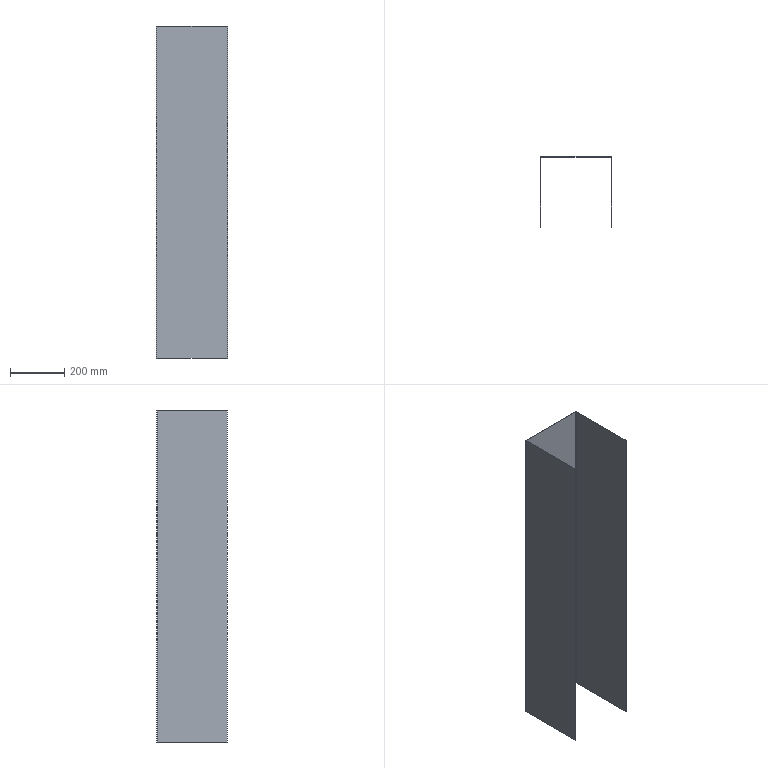Part | 1 solid | 22 faces | box 262 x 261 x 1225 mm | volume 956650 mm3 | plane 18 | cylinder 4 | commonest cylinder face diameters 1.473 x2 3.473 x2
STEP:
#1=CARTESIAN_POINT('',(129.263,260.,1225.));
#2=VERTEX_POINT('',#1);
#3=CARTESIAN_POINT('',(129.263,261.,1225.));
#4=VERTEX_POINT('',#3);
#5=CARTESIAN_POINT('',(129.263,260.,1225.));
#6=DIRECTION('',(0.,1.,0.));
#7=VECTOR('',#6,1000.);
#8=LINE('',#5,#7);
#9=EDGE_CURVE('',#2,#4,#8,.T.);
#10=ORIENTED_EDGE('',*,*,#9,.F.);
#11=CARTESIAN_POINT('',(130.,259.263,1225.));
#12=VERTEX_POINT('',#11);
#13=CARTESIAN_POINT('',(129.263,259.263,1225.));
#14=DIRECTION('',(0.,0.,1.));
#15=DIRECTION('',(-1.,0.,0.));
#16=AXIS2_PLACEMENT_3D('',#13,#14,#15);
#17=CIRCLE('',#16,0.7366);
#18=EDGE_CURVE('',#12,#2,#17,.T.);
#19=ORIENTED_EDGE('',*,*,#18,.F.);
#20=CARTESIAN_POINT('',(131.,259.263,1225.));
#21=VERTEX_POINT('',#20);
#22=CARTESIAN_POINT('',(131.,259.263,1225.));
#23=DIRECTION('',(-1.,0.,0.));
#24=VECTOR('',#23,1000.);
#25=LINE('',#22,#24);
#26=EDGE_CURVE('',#21,#12,#25,.T.);
#27=ORIENTED_EDGE('',*,*,#26,.F.);
#28=CARTESIAN_POINT('',(129.263,259.263,1225.));
#29=DIRECTION('',(0.,0.,1.));
#30=DIRECTION('',(1.,0.,0.));
#31=AXIS2_PLACEMENT_3D('',#28,#29,#30);
#32=CIRCLE('',#31,1.737);
#33=EDGE_CURVE('',#21,#4,#32,.T.);
#34=ORIENTED_EDGE('',*,*,#33,.T.);
#35=EDGE_LOOP('',(#10,#19,#27,#34));
#36=FACE_OUTER_BOUND('',#35,.T.);
#37=CARTESIAN_POINT('',(129.263,260.,1225.));
#38=DIRECTION('',(0.,0.,1.));
#39=DIRECTION('',(1.,0.,0.));
#40=AXIS2_PLACEMENT_3D('',#37,#38,#39);
#41=PLANE('',#40);
#42=ADVANCED_FACE('',(#36),#41,.T.);
#43=CARTESIAN_POINT('',(-129.263,260.,1225.));
#44=VERTEX_POINT('',#43);
#45=CARTESIAN_POINT('',(-130.,260.,1225.));
#46=DIRECTION('',(-1.,0.,0.));
#47=VECTOR('',#46,1000.);
#48=LINE('',#45,#47);
#49=EDGE_CURVE('',#2,#44,#48,.T.);
#50=ORIENTED_EDGE('',*,*,#49,.F.);
#51=ORIENTED_EDGE('',*,*,#9,.T.);
#52=CARTESIAN_POINT('',(-129.263,261.,1225.));
#53=VERTEX_POINT('',#52);
#54=CARTESIAN_POINT('',(-130.,261.,1225.));
#55=DIRECTION('',(-1.,0.,0.));
#56=VECTOR('',#55,1000.);
#57=LINE('',#54,#56);
#58=EDGE_CURVE('',#4,#53,#57,.T.);
#59=ORIENTED_EDGE('',*,*,#58,.T.);
#60=CARTESIAN_POINT('',(-129.263,261.,1225.));
#61=DIRECTION('',(0.,-1.,0.));
#62=VECTOR('',#61,1000.);
#63=LINE('',#60,#62);
#64=EDGE_CURVE('',#53,#44,#63,.T.);
#65=ORIENTED_EDGE('',*,*,#64,.T.);
#66=EDGE_LOOP('',(#50,#51,#59,#65));
#67=FACE_OUTER_BOUND('',#66,.T.);
#68=CARTESIAN_POINT('',(131.,259.263,1225.));
#69=DIRECTION('',(0.,0.,1.));
#70=DIRECTION('',(1.,0.,0.));
#71=AXIS2_PLACEMENT_3D('',#68,#69,#70);
#72=PLANE('',#71);
#73=ADVANCED_FACE('',(#67),#72,.T.);
#74=CARTESIAN_POINT('',(130.,259.263,0.));
#75=VERTEX_POINT('',#74);
#76=CARTESIAN_POINT('',(131.,259.263,0.));
#77=VERTEX_POINT('',#76);
#78=CARTESIAN_POINT('',(130.,259.263,0.));
#79=DIRECTION('',(1.,0.,0.));
#80=VECTOR('',#79,1000.);
#81=LINE('',#78,#80);
#82=EDGE_CURVE('',#75,#77,#81,.T.);
#83=ORIENTED_EDGE('',*,*,#82,.F.);
#84=CARTESIAN_POINT('',(129.263,260.,0.));
#85=VERTEX_POINT('',#84);
#86=CARTESIAN_POINT('',(129.263,259.263,0.));
#87=DIRECTION('',(0.,0.,1.));
#88=DIRECTION('',(-1.,0.,0.));
#89=AXIS2_PLACEMENT_3D('',#86,#87,#88);
#90=CIRCLE('',#89,0.7366);
#91=EDGE_CURVE('',#75,#85,#90,.T.);
#92=ORIENTED_EDGE('',*,*,#91,.T.);
#93=CARTESIAN_POINT('',(129.263,261.,0.));
#94=VERTEX_POINT('',#93);
#95=CARTESIAN_POINT('',(129.263,261.,0.));
#96=DIRECTION('',(0.,-1.,0.));
#97=VECTOR('',#96,1000.);
#98=LINE('',#95,#97);
#99=EDGE_CURVE('',#94,#85,#98,.T.);
#100=ORIENTED_EDGE('',*,*,#99,.F.);
#101=CARTESIAN_POINT('',(129.263,259.263,0.));
#102=DIRECTION('',(0.,0.,1.));
#103=DIRECTION('',(1.,0.,0.));
#104=AXIS2_PLACEMENT_3D('',#101,#102,#103);
#105=CIRCLE('',#104,1.737);
#106=EDGE_CURVE('',#77,#94,#105,.T.);
#107=ORIENTED_EDGE('',*,*,#106,.F.);
#108=EDGE_LOOP('',(#83,#92,#100,#107));
#109=FACE_OUTER_BOUND('',#108,.T.);
#110=CARTESIAN_POINT('',(130.,259.263,0.));
#111=DIRECTION('',(0.,0.,-1.));
#112=DIRECTION('',(-1.,0.,0.));
#113=AXIS2_PLACEMENT_3D('',#110,#111,#112);
#114=PLANE('',#113);
#115=ADVANCED_FACE('',(#109),#114,.T.);
#116=CARTESIAN_POINT('',(130.,0.,0.));
#117=VERTEX_POINT('',#116);
#118=CARTESIAN_POINT('',(130.,260.,0.));
#119=DIRECTION('',(0.,1.,0.));
#120=VECTOR('',#119,1000.);
#121=LINE('',#118,#120);
#122=EDGE_CURVE('',#117,#75,#121,.T.);
#123=ORIENTED_EDGE('',*,*,#122,.T.);
#124=ORIENTED_EDGE('',*,*,#82,.T.);
#125=CARTESIAN_POINT('',(131.,0.,0.));
#126=VERTEX_POINT('',#125);
#127=CARTESIAN_POINT('',(131.,260.,0.));
#128=DIRECTION('',(0.,1.,0.));
#129=VECTOR('',#128,1000.);
#130=LINE('',#127,#129);
#131=EDGE_CURVE('',#126,#77,#130,.T.);
#132=ORIENTED_EDGE('',*,*,#131,.F.);
#133=CARTESIAN_POINT('',(131.,0.,0.));
#134=DIRECTION('',(-1.,0.,0.));
#135=VECTOR('',#134,1000.);
#136=LINE('',#133,#135);
#137=EDGE_CURVE('',#126,#117,#136,.T.);
#138=ORIENTED_EDGE('',*,*,#137,.T.);
#139=EDGE_LOOP('',(#123,#124,#132,#138));
#140=FACE_OUTER_BOUND('',#139,.T.);
#141=CARTESIAN_POINT('',(129.263,261.,0.));
#142=DIRECTION('',(0.,0.,-1.));
#143=DIRECTION('',(-1.,0.,0.));
#144=AXIS2_PLACEMENT_3D('',#141,#142,#143);
#145=PLANE('',#144);
#146=ADVANCED_FACE('',(#140),#145,.T.);
#147=CARTESIAN_POINT('',(-130.,259.263,1225.));
#148=VERTEX_POINT('',#147);
#149=CARTESIAN_POINT('',(-131.,259.263,1225.));
#150=VERTEX_POINT('',#149);
#151=CARTESIAN_POINT('',(-130.,259.263,1225.));
#152=DIRECTION('',(-1.,0.,0.));
#153=VECTOR('',#152,1000.);
#154=LINE('',#151,#153);
#155=EDGE_CURVE('',#148,#150,#154,.T.);
#156=ORIENTED_EDGE('',*,*,#155,.F.);
#157=CARTESIAN_POINT('',(-129.263,259.263,1225.));
#158=DIRECTION('',(0.,0.,1.));
#159=DIRECTION('',(-1.,0.,0.));
#160=AXIS2_PLACEMENT_3D('',#157,#158,#159);
#161=CIRCLE('',#160,0.7366);
#162=EDGE_CURVE('',#44,#148,#161,.T.);
#163=ORIENTED_EDGE('',*,*,#162,.F.);
#164=ORIENTED_EDGE('',*,*,#64,.F.);
#165=CARTESIAN_POINT('',(-129.263,259.263,1225.));
#166=DIRECTION('',(0.,0.,1.));
#167=DIRECTION('',(1.,0.,0.));
#168=AXIS2_PLACEMENT_3D('',#165,#166,#167);
#169=CIRCLE('',#168,1.737);
#170=EDGE_CURVE('',#53,#150,#169,.T.);
#171=ORIENTED_EDGE('',*,*,#170,.T.);
#172=EDGE_LOOP('',(#156,#163,#164,#171));
#173=FACE_OUTER_BOUND('',#172,.T.);
#174=CARTESIAN_POINT('',(-130.,259.263,1225.));
#175=DIRECTION('',(0.,0.,1.));
#176=DIRECTION('',(1.,0.,0.));
#177=AXIS2_PLACEMENT_3D('',#174,#175,#176);
#178=PLANE('',#177);
#179=ADVANCED_FACE('',(#173),#178,.T.);
#180=CARTESIAN_POINT('',(-130.,0.,1225.));
#181=VERTEX_POINT('',#180);
#182=CARTESIAN_POINT('',(-130.,260.,1225.));
#183=DIRECTION('',(0.,-1.,0.));
#184=VECTOR('',#183,1000.);
#185=LINE('',#182,#184);
#186=EDGE_CURVE('',#148,#181,#185,.T.);
#187=ORIENTED_EDGE('',*,*,#186,.F.);
#188=ORIENTED_EDGE('',*,*,#155,.T.);
#189=CARTESIAN_POINT('',(-131.,0.,1225.));
#190=VERTEX_POINT('',#189);
#191=CARTESIAN_POINT('',(-131.,260.,1225.));
#192=DIRECTION('',(0.,-1.,0.));
#193=VECTOR('',#192,1000.);
#194=LINE('',#191,#193);
#195=EDGE_CURVE('',#150,#190,#194,.T.);
#196=ORIENTED_EDGE('',*,*,#195,.T.);
#197=CARTESIAN_POINT('',(-130.,0.,1225.));
#198=DIRECTION('',(-1.,0.,0.));
#199=VECTOR('',#198,1000.);
#200=LINE('',#197,#199);
#201=EDGE_CURVE('',#181,#190,#200,.T.);
#202=ORIENTED_EDGE('',*,*,#201,.F.);
#203=EDGE_LOOP('',(#187,#188,#196,#202));
#204=FACE_OUTER_BOUND('',#203,.T.);
#205=CARTESIAN_POINT('',(-129.263,261.,1225.));
#206=DIRECTION('',(0.,0.,1.));
#207=DIRECTION('',(1.,0.,0.));
#208=AXIS2_PLACEMENT_3D('',#205,#206,#207);
#209=PLANE('',#208);
#210=ADVANCED_FACE('',(#204),#209,.T.);
#211=CARTESIAN_POINT('',(-129.263,260.,0.));
#212=VERTEX_POINT('',#211);
#213=CARTESIAN_POINT('',(-129.263,261.,0.));
#214=VERTEX_POINT('',#213);
#215=CARTESIAN_POINT('',(-129.263,260.,0.));
#216=DIRECTION('',(0.,1.,0.));
#217=VECTOR('',#216,1000.);
#218=LINE('',#215,#217);
#219=EDGE_CURVE('',#212,#214,#218,.T.);
#220=ORIENTED_EDGE('',*,*,#219,.F.);
#221=CARTESIAN_POINT('',(-130.,259.263,0.));
#222=VERTEX_POINT('',#221);
#223=CARTESIAN_POINT('',(-129.263,259.263,0.));
#224=DIRECTION('',(0.,0.,1.));
#225=DIRECTION('',(-1.,0.,0.));
#226=AXIS2_PLACEMENT_3D('',#223,#224,#225);
#227=CIRCLE('',#226,0.7366);
#228=EDGE_CURVE('',#212,#222,#227,.T.);
#229=ORIENTED_EDGE('',*,*,#228,.T.);
#230=CARTESIAN_POINT('',(-131.,259.263,0.));
#231=VERTEX_POINT('',#230);
#232=CARTESIAN_POINT('',(-131.,259.263,0.));
#233=DIRECTION('',(1.,0.,0.));
#234=VECTOR('',#233,1000.);
#235=LINE('',#232,#234);
#236=EDGE_CURVE('',#231,#222,#235,.T.);
#237=ORIENTED_EDGE('',*,*,#236,.F.);
#238=CARTESIAN_POINT('',(-129.263,259.263,0.));
#239=DIRECTION('',(0.,0.,1.));
#240=DIRECTION('',(1.,0.,0.));
#241=AXIS2_PLACEMENT_3D('',#238,#239,#240);
#242=CIRCLE('',#241,1.737);
#243=EDGE_CURVE('',#214,#231,#242,.T.);
#244=ORIENTED_EDGE('',*,*,#243,.F.);
#245=EDGE_LOOP('',(#220,#229,#237,#244));
#246=FACE_OUTER_BOUND('',#245,.T.);
#247=CARTESIAN_POINT('',(-129.263,260.,0.));
#248=DIRECTION('',(0.,0.,-1.));
#249=DIRECTION('',(-1.,0.,0.));
#250=AXIS2_PLACEMENT_3D('',#247,#248,#249);
#251=PLANE('',#250);
#252=ADVANCED_FACE('',(#246),#251,.T.);
#253=CARTESIAN_POINT('',(-130.,260.,0.));
#254=DIRECTION('',(-1.,0.,0.));
#255=VECTOR('',#254,1000.);
#256=LINE('',#253,#255);
#257=EDGE_CURVE('',#85,#212,#256,.T.);
#258=ORIENTED_EDGE('',*,*,#257,.T.);
#259=ORIENTED_EDGE('',*,*,#219,.T.);
#260=CARTESIAN_POINT('',(-130.,261.,0.));
#261=DIRECTION('',(-1.,0.,0.));
#262=VECTOR('',#261,1000.);
#263=LINE('',#260,#262);
#264=EDGE_CURVE('',#94,#214,#263,.T.);
#265=ORIENTED_EDGE('',*,*,#264,.F.);
#266=ORIENTED_EDGE('',*,*,#99,.T.);
#267=EDGE_LOOP('',(#258,#259,#265,#266));
#268=FACE_OUTER_BOUND('',#267,.T.);
#269=CARTESIAN_POINT('',(-131.,259.263,0.));
#270=DIRECTION('',(0.,0.,-1.));
#271=DIRECTION('',(-1.,0.,0.));
#272=AXIS2_PLACEMENT_3D('',#269,#270,#271);
#273=PLANE('',#272);
#274=ADVANCED_FACE('',(#268),#273,.T.);
#275=CARTESIAN_POINT('',(-131.,0.,0.));
#276=VERTEX_POINT('',#275);
#277=CARTESIAN_POINT('',(-131.,260.,0.));
#278=DIRECTION('',(0.,-1.,0.));
#279=VECTOR('',#278,1000.);
#280=LINE('',#277,#279);
#281=EDGE_CURVE('',#231,#276,#280,.T.);
#282=ORIENTED_EDGE('',*,*,#281,.T.);
#283=CARTESIAN_POINT('',(-131.,0.,1225.));
#284=DIRECTION('',(0.,0.,-1.));
#285=VECTOR('',#284,1000.);
#286=LINE('',#283,#285);
#287=EDGE_CURVE('',#190,#276,#286,.T.);
#288=ORIENTED_EDGE('',*,*,#287,.F.);
#289=ORIENTED_EDGE('',*,*,#195,.F.);
#290=CARTESIAN_POINT('',(-131.,259.263,1225.));
#291=DIRECTION('',(0.,0.,-1.));
#292=VECTOR('',#291,1000.);
#293=LINE('',#290,#292);
#294=EDGE_CURVE('',#150,#231,#293,.T.);
#295=ORIENTED_EDGE('',*,*,#294,.T.);
#296=EDGE_LOOP('',(#282,#288,#289,#295));
#297=FACE_OUTER_BOUND('',#296,.T.);
#298=CARTESIAN_POINT('',(-131.,260.,1225.));
#299=DIRECTION('',(1.,0.,0.));
#300=DIRECTION('',(0.,0.,-1.));
#301=AXIS2_PLACEMENT_3D('',#298,#299,#300);
#302=PLANE('',#301);
#303=ADVANCED_FACE('',(#297),#302,.F.);
#304=CARTESIAN_POINT('',(-130.,0.,0.));
#305=VERTEX_POINT('',#304);
#306=CARTESIAN_POINT('',(-130.,0.,0.));
#307=DIRECTION('',(-1.,0.,0.));
#308=VECTOR('',#307,1000.);
#309=LINE('',#306,#308);
#310=EDGE_CURVE('',#305,#276,#309,.T.);
#311=ORIENTED_EDGE('',*,*,#310,.F.);
#312=CARTESIAN_POINT('',(-130.,0.,1225.));
#313=DIRECTION('',(0.,0.,-1.));
#314=VECTOR('',#313,1000.);
#315=LINE('',#312,#314);
#316=EDGE_CURVE('',#181,#305,#315,.T.);
#317=ORIENTED_EDGE('',*,*,#316,.F.);
#318=ORIENTED_EDGE('',*,*,#201,.T.);
#319=ORIENTED_EDGE('',*,*,#287,.T.);
#320=EDGE_LOOP('',(#311,#317,#318,#319));
#321=FACE_OUTER_BOUND('',#320,.T.);
#322=CARTESIAN_POINT('',(-130.,0.,1225.));
#323=DIRECTION('',(0.,-1.,0.));
#324=DIRECTION('',(1.,0.,0.));
#325=AXIS2_PLACEMENT_3D('',#322,#323,#324);
#326=PLANE('',#325);
#327=ADVANCED_FACE('',(#321),#326,.T.);
#328=CARTESIAN_POINT('',(-130.,260.,0.));
#329=DIRECTION('',(0.,-1.,0.));
#330=VECTOR('',#329,1000.);
#331=LINE('',#328,#330);
#332=EDGE_CURVE('',#222,#305,#331,.T.);
#333=ORIENTED_EDGE('',*,*,#332,.F.);
#334=CARTESIAN_POINT('',(-130.,259.263,1225.));
#335=DIRECTION('',(0.,0.,-1.));
#336=VECTOR('',#335,1000.);
#337=LINE('',#334,#336);
#338=EDGE_CURVE('',#148,#222,#337,.T.);
#339=ORIENTED_EDGE('',*,*,#338,.F.);
#340=ORIENTED_EDGE('',*,*,#186,.T.);
#341=ORIENTED_EDGE('',*,*,#316,.T.);
#342=EDGE_LOOP('',(#333,#339,#340,#341));
#343=FACE_OUTER_BOUND('',#342,.T.);
#344=CARTESIAN_POINT('',(-130.,260.,1225.));
#345=DIRECTION('',(1.,0.,0.));
#346=DIRECTION('',(0.,0.,-1.));
#347=AXIS2_PLACEMENT_3D('',#344,#345,#346);
#348=PLANE('',#347);
#349=ADVANCED_FACE('',(#343),#348,.T.);
#350=ORIENTED_EDGE('',*,*,#228,.F.);
#351=CARTESIAN_POINT('',(-129.263,260.,1225.));
#352=DIRECTION('',(0.,0.,-1.));
#353=VECTOR('',#352,1000.);
#354=LINE('',#351,#353);
#355=EDGE_CURVE('',#44,#212,#354,.T.);
#356=ORIENTED_EDGE('',*,*,#355,.F.);
#357=ORIENTED_EDGE('',*,*,#162,.T.);
#358=ORIENTED_EDGE('',*,*,#338,.T.);
#359=EDGE_LOOP('',(#350,#356,#357,#358));
#360=FACE_OUTER_BOUND('',#359,.T.);
#361=CARTESIAN_POINT('',(-129.263,259.263,1225.));
#362=DIRECTION('',(0.,0.,-1.));
#363=DIRECTION('',(-1.,0.,0.));
#364=AXIS2_PLACEMENT_3D('',#361,#362,#363);
#365=CYLINDRICAL_SURFACE('',#364,0.7366);
#366=ADVANCED_FACE('',(#360),#365,.F.);
#367=ORIENTED_EDGE('',*,*,#257,.F.);
#368=CARTESIAN_POINT('',(129.263,260.,1225.));
#369=DIRECTION('',(0.,0.,-1.));
#370=VECTOR('',#369,1000.);
#371=LINE('',#368,#370);
#372=EDGE_CURVE('',#2,#85,#371,.T.);
#373=ORIENTED_EDGE('',*,*,#372,.F.);
#374=ORIENTED_EDGE('',*,*,#49,.T.);
#375=ORIENTED_EDGE('',*,*,#355,.T.);
#376=EDGE_LOOP('',(#367,#373,#374,#375));
#377=FACE_OUTER_BOUND('',#376,.T.);
#378=CARTESIAN_POINT('',(-130.,260.,1225.));
#379=DIRECTION('',(0.,-1.,0.));
#380=DIRECTION('',(0.,0.,-1.));
#381=AXIS2_PLACEMENT_3D('',#378,#379,#380);
#382=PLANE('',#381);
#383=ADVANCED_FACE('',(#377),#382,.T.);
#384=ORIENTED_EDGE('',*,*,#91,.F.);
#385=CARTESIAN_POINT('',(130.,259.263,1225.));
#386=DIRECTION('',(0.,0.,-1.));
#387=VECTOR('',#386,1000.);
#388=LINE('',#385,#387);
#389=EDGE_CURVE('',#12,#75,#388,.T.);
#390=ORIENTED_EDGE('',*,*,#389,.F.);
#391=ORIENTED_EDGE('',*,*,#18,.T.);
#392=ORIENTED_EDGE('',*,*,#372,.T.);
#393=EDGE_LOOP('',(#384,#390,#391,#392));
#394=FACE_OUTER_BOUND('',#393,.T.);
#395=CARTESIAN_POINT('',(129.263,259.263,1225.));
#396=DIRECTION('',(0.,0.,-1.));
#397=DIRECTION('',(-1.,0.,0.));
#398=AXIS2_PLACEMENT_3D('',#395,#396,#397);
#399=CYLINDRICAL_SURFACE('',#398,0.7366);
#400=ADVANCED_FACE('',(#394),#399,.F.);
#401=ORIENTED_EDGE('',*,*,#122,.F.);
#402=CARTESIAN_POINT('',(130.,0.,1225.));
#403=VERTEX_POINT('',#402);
#404=CARTESIAN_POINT('',(130.,0.,1225.));
#405=DIRECTION('',(0.,0.,-1.));
#406=VECTOR('',#405,1000.);
#407=LINE('',#404,#406);
#408=EDGE_CURVE('',#403,#117,#407,.T.);
#409=ORIENTED_EDGE('',*,*,#408,.F.);
#410=CARTESIAN_POINT('',(130.,260.,1225.));
#411=DIRECTION('',(0.,1.,0.));
#412=VECTOR('',#411,1000.);
#413=LINE('',#410,#412);
#414=EDGE_CURVE('',#403,#12,#413,.T.);
#415=ORIENTED_EDGE('',*,*,#414,.T.);
#416=ORIENTED_EDGE('',*,*,#389,.T.);
#417=EDGE_LOOP('',(#401,#409,#415,#416));
#418=FACE_OUTER_BOUND('',#417,.T.);
#419=CARTESIAN_POINT('',(130.,260.,1225.));
#420=DIRECTION('',(-1.,0.,0.));
#421=DIRECTION('',(0.,0.,1.));
#422=AXIS2_PLACEMENT_3D('',#419,#420,#421);
#423=PLANE('',#422);
#424=ADVANCED_FACE('',(#418),#423,.T.);
#425=ORIENTED_EDGE('',*,*,#137,.F.);
#426=CARTESIAN_POINT('',(131.,0.,1225.));
#427=VERTEX_POINT('',#426);
#428=CARTESIAN_POINT('',(131.,0.,1225.));
#429=DIRECTION('',(0.,0.,-1.));
#430=VECTOR('',#429,1000.);
#431=LINE('',#428,#430);
#432=EDGE_CURVE('',#427,#126,#431,.T.);
#433=ORIENTED_EDGE('',*,*,#432,.F.);
#434=CARTESIAN_POINT('',(131.,0.,1225.));
#435=DIRECTION('',(-1.,0.,0.));
#436=VECTOR('',#435,1000.);
#437=LINE('',#434,#436);
#438=EDGE_CURVE('',#427,#403,#437,.T.);
#439=ORIENTED_EDGE('',*,*,#438,.T.);
#440=ORIENTED_EDGE('',*,*,#408,.T.);
#441=EDGE_LOOP('',(#425,#433,#439,#440));
#442=FACE_OUTER_BOUND('',#441,.T.);
#443=CARTESIAN_POINT('',(131.,0.,1225.));
#444=DIRECTION('',(0.,-1.,0.));
#445=DIRECTION('',(1.,0.,0.));
#446=AXIS2_PLACEMENT_3D('',#443,#444,#445);
#447=PLANE('',#446);
#448=ADVANCED_FACE('',(#442),#447,.T.);
#449=ORIENTED_EDGE('',*,*,#131,.T.);
#450=CARTESIAN_POINT('',(131.,259.263,1225.));
#451=DIRECTION('',(0.,0.,-1.));
#452=VECTOR('',#451,1000.);
#453=LINE('',#450,#452);
#454=EDGE_CURVE('',#21,#77,#453,.T.);
#455=ORIENTED_EDGE('',*,*,#454,.F.);
#456=CARTESIAN_POINT('',(131.,260.,1225.));
#457=DIRECTION('',(0.,1.,0.));
#458=VECTOR('',#457,1000.);
#459=LINE('',#456,#458);
#460=EDGE_CURVE('',#427,#21,#459,.T.);
#461=ORIENTED_EDGE('',*,*,#460,.F.);
#462=ORIENTED_EDGE('',*,*,#432,.T.);
#463=EDGE_LOOP('',(#449,#455,#461,#462));
#464=FACE_OUTER_BOUND('',#463,.T.);
#465=CARTESIAN_POINT('',(131.,260.,1225.));
#466=DIRECTION('',(-1.,0.,0.));
#467=DIRECTION('',(0.,0.,1.));
#468=AXIS2_PLACEMENT_3D('',#465,#466,#467);
#469=PLANE('',#468);
#470=ADVANCED_FACE('',(#464),#469,.F.);
#471=ORIENTED_EDGE('',*,*,#106,.T.);
#472=CARTESIAN_POINT('',(129.263,261.,1225.));
#473=DIRECTION('',(0.,0.,-1.));
#474=VECTOR('',#473,1000.);
#475=LINE('',#472,#474);
#476=EDGE_CURVE('',#4,#94,#475,.T.);
#477=ORIENTED_EDGE('',*,*,#476,.F.);
#478=ORIENTED_EDGE('',*,*,#33,.F.);
#479=ORIENTED_EDGE('',*,*,#454,.T.);
#480=EDGE_LOOP('',(#471,#477,#478,#479));
#481=FACE_OUTER_BOUND('',#480,.T.);
#482=CARTESIAN_POINT('',(129.263,259.263,1225.));
#483=DIRECTION('',(0.,0.,-1.));
#484=DIRECTION('',(-1.,0.,0.));
#485=AXIS2_PLACEMENT_3D('',#482,#483,#484);
#486=CYLINDRICAL_SURFACE('',#485,1.737);
#487=ADVANCED_FACE('',(#481),#486,.T.);
#488=ORIENTED_EDGE('',*,*,#264,.T.);
#489=CARTESIAN_POINT('',(-129.263,261.,1225.));
#490=DIRECTION('',(0.,0.,-1.));
#491=VECTOR('',#490,1000.);
#492=LINE('',#489,#491);
#493=EDGE_CURVE('',#53,#214,#492,.T.);
#494=ORIENTED_EDGE('',*,*,#493,.F.);
#495=ORIENTED_EDGE('',*,*,#58,.F.);
#496=ORIENTED_EDGE('',*,*,#476,.T.);
#497=EDGE_LOOP('',(#488,#494,#495,#496));
#498=FACE_OUTER_BOUND('',#497,.T.);
#499=CARTESIAN_POINT('',(-130.,261.,1225.));
#500=DIRECTION('',(0.,-1.,0.));
#501=DIRECTION('',(0.,0.,-1.));
#502=AXIS2_PLACEMENT_3D('',#499,#500,#501);
#503=PLANE('',#502);
#504=ADVANCED_FACE('',(#498),#503,.F.);
#505=ORIENTED_EDGE('',*,*,#243,.T.);
#506=ORIENTED_EDGE('',*,*,#294,.F.);
#507=ORIENTED_EDGE('',*,*,#170,.F.);
#508=ORIENTED_EDGE('',*,*,#493,.T.);
#509=EDGE_LOOP('',(#505,#506,#507,#508));
#510=FACE_OUTER_BOUND('',#509,.T.);
#511=CARTESIAN_POINT('',(-129.263,259.263,1225.));
#512=DIRECTION('',(0.,0.,-1.));
#513=DIRECTION('',(-1.,0.,0.));
#514=AXIS2_PLACEMENT_3D('',#511,#512,#513);
#515=CYLINDRICAL_SURFACE('',#514,1.737);
#516=ADVANCED_FACE('',(#510),#515,.T.);
#517=ORIENTED_EDGE('',*,*,#460,.T.);
#518=ORIENTED_EDGE('',*,*,#26,.T.);
#519=ORIENTED_EDGE('',*,*,#414,.F.);
#520=ORIENTED_EDGE('',*,*,#438,.F.);
#521=EDGE_LOOP('',(#517,#518,#519,#520));
#522=FACE_OUTER_BOUND('',#521,.T.);
#523=CARTESIAN_POINT('',(-129.263,259.263,1225.));
#524=DIRECTION('',(0.,0.,-1.));
#525=DIRECTION('',(-1.,0.,0.));
#526=AXIS2_PLACEMENT_3D('',#523,#524,#525);
#527=PLANE('',#526);
#528=ADVANCED_FACE('',(#522),#527,.F.);
#529=ORIENTED_EDGE('',*,*,#281,.F.);
#530=ORIENTED_EDGE('',*,*,#236,.T.);
#531=ORIENTED_EDGE('',*,*,#332,.T.);
#532=ORIENTED_EDGE('',*,*,#310,.T.);
#533=EDGE_LOOP('',(#529,#530,#531,#532));
#534=FACE_OUTER_BOUND('',#533,.T.);
#535=CARTESIAN_POINT('',(-129.263,259.263,0.));
#536=DIRECTION('',(0.,0.,-1.));
#537=DIRECTION('',(-1.,0.,0.));
#538=AXIS2_PLACEMENT_3D('',#535,#536,#537);
#539=PLANE('',#538);
#540=ADVANCED_FACE('',(#534),#539,.T.);
#541=CLOSED_SHELL('',(#42,#73,#115,#146,#179,#210,#252,#274,#303,#327,#349,#366,#383,#400,#424,#448,#470,#487,#504,#516,#528,#540));
#542=MANIFOLD_SOLID_BREP('',#541);
#543=CARTESIAN_POINT('',(0.,0.,0.));
#544=DIRECTION('',(0.,0.,1.));
#545=DIRECTION('',(1.,0.,0.));
#546=AXIS2_PLACEMENT_3D('',#543,#544,#545);
#547=(LENGTH_UNIT()NAMED_UNIT(*)SI_UNIT(.MILLI.,.METRE.));
#548=UNCERTAINTY_MEASURE_WITH_UNIT(LENGTH_MEASURE(0.00001),#547,'','');
#549=(NAMED_UNIT(*)PLANE_ANGLE_UNIT()SI_UNIT($,.RADIAN.));
#550=(NAMED_UNIT(*)SI_UNIT($,.STERADIAN.)SOLID_ANGLE_UNIT());
#551=(GEOMETRIC_REPRESENTATION_CONTEXT(3)GLOBAL_UNCERTAINTY_ASSIGNED_CONTEXT((#548))GLOBAL_UNIT_ASSIGNED_CONTEXT((#547,#549,#550))REPRESENTATION_CONTEXT('',''));
#552=ADVANCED_BREP_SHAPE_REPRESENTATION('',(#542,#546),#551);